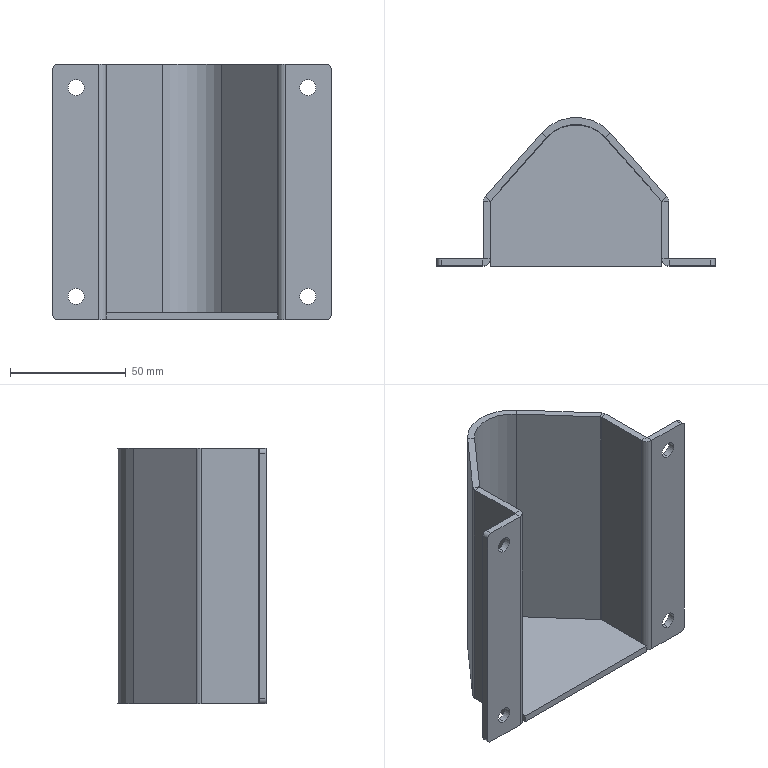Part | SolidWorks | features FlatPattern 2, SMBaseFlange 2, SheetMetal 2, Fillet 1, ICE 1 | 2 solids | 68 faces | box 120 x 64 x 110 mm | volume 76419 mm3 | plane 43 | cylinder 25 | commonest cylinder face diameters 7 x8 0.4 x6 4 x4 6.4 x4 34 x2 40 x1